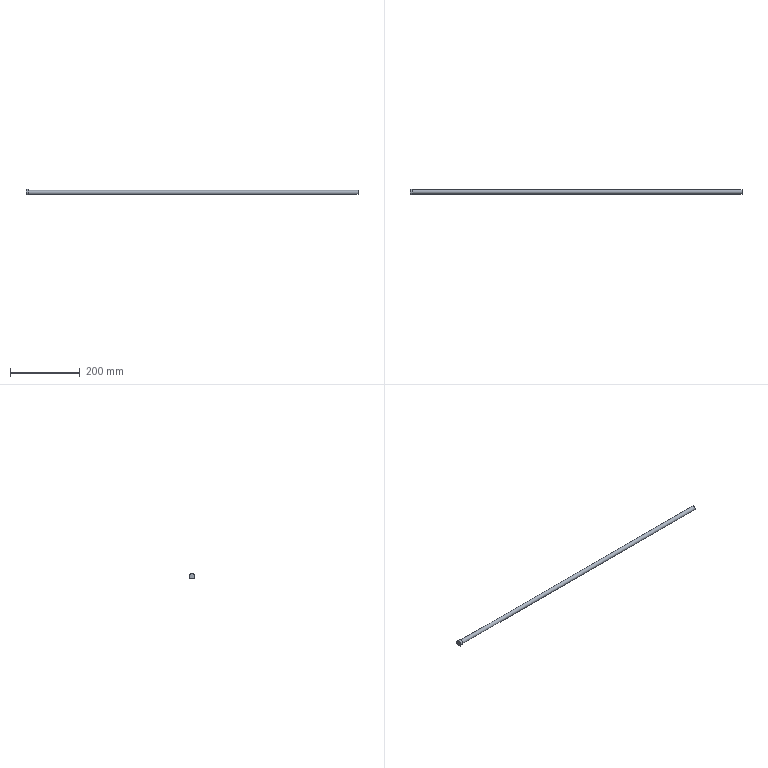Part | STEP file | solid 43 | 1 solid | 6 faces | box 955 x 17 x 15 mm | volume 108799 mm3 | plane 4 | cylinder 2 | commonest cylinder face diameters 12 x1 17 x1